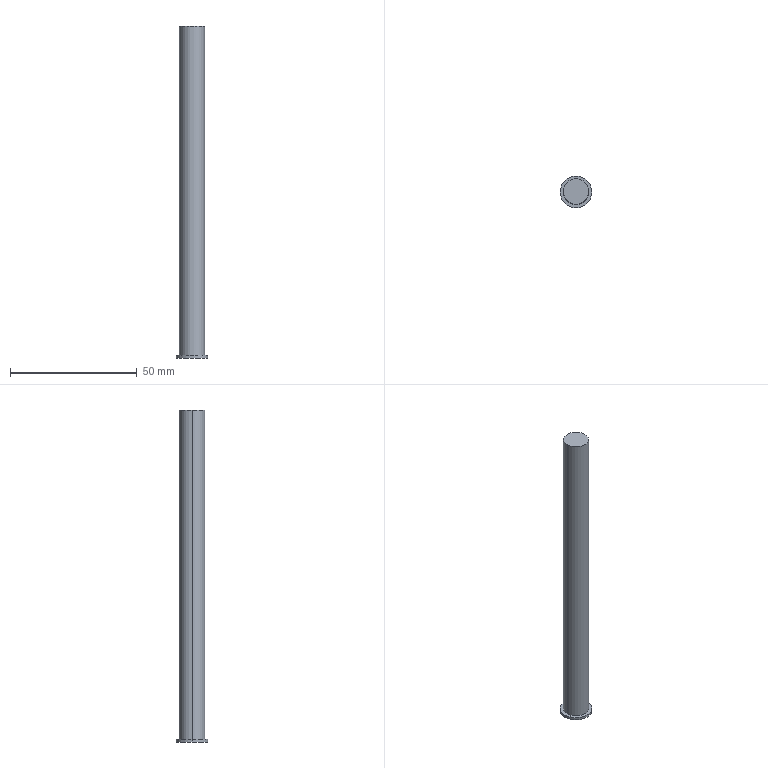Part | SolidWorks | features Extrusion 1, ICE 1 | 1 solid | 7 faces | box 12.5 x 12.5 x 131 mm | volume 10333 mm3 | cylinder 4 | plane 3 | commonest cylinder face diameters 10 x2 12.5 x2
STEP:
#1=CARTESIAN_POINT('',(-6.25,0.,-1.));
#2=VERTEX_POINT('',#1);
#3=CARTESIAN_POINT('',(6.25,0.,-1.));
#4=VERTEX_POINT('',#3);
#5=CARTESIAN_POINT('',(0.,0.,-1.));
#6=DIRECTION('',(0.,0.,-1.));
#7=DIRECTION('',(-1.,0.,0.));
#8=AXIS2_PLACEMENT_3D('',#5,#6,#7);
#9=CIRCLE('',#8,6.25);
#10=EDGE_CURVE('',#2,#4,#9,.T.);
#11=ORIENTED_EDGE('',*,*,#10,.F.);
#12=CARTESIAN_POINT('',(-6.25,0.,0.));
#13=VERTEX_POINT('',#12);
#14=CARTESIAN_POINT('',(-6.25,0.,-1.));
#15=DIRECTION('',(0.,0.,1.));
#16=VECTOR('',#15,1000.);
#17=LINE('',#14,#16);
#18=EDGE_CURVE('',#2,#13,#17,.T.);
#19=ORIENTED_EDGE('',*,*,#18,.T.);
#20=CARTESIAN_POINT('',(6.25,0.,0.));
#21=VERTEX_POINT('',#20);
#22=CARTESIAN_POINT('',(0.,0.,0.));
#23=DIRECTION('',(0.,0.,-1.));
#24=DIRECTION('',(-1.,0.,0.));
#25=AXIS2_PLACEMENT_3D('',#22,#23,#24);
#26=CIRCLE('',#25,6.25);
#27=EDGE_CURVE('',#13,#21,#26,.T.);
#28=ORIENTED_EDGE('',*,*,#27,.T.);
#29=CARTESIAN_POINT('',(6.25,0.,-1.));
#30=DIRECTION('',(0.,0.,1.));
#31=VECTOR('',#30,1000.);
#32=LINE('',#29,#31);
#33=EDGE_CURVE('',#4,#21,#32,.T.);
#34=ORIENTED_EDGE('',*,*,#33,.F.);
#35=EDGE_LOOP('',(#11,#19,#28,#34));
#36=FACE_OUTER_BOUND('',#35,.T.);
#37=CARTESIAN_POINT('',(0.,0.,-1.));
#38=DIRECTION('',(0.,0.,1.));
#39=DIRECTION('',(1.,0.,0.));
#40=AXIS2_PLACEMENT_3D('',#37,#38,#39);
#41=CYLINDRICAL_SURFACE('',#40,6.25);
#42=ADVANCED_FACE('',(#36),#41,.T.);
#43=CARTESIAN_POINT('',(5.,0.,130.));
#44=VERTEX_POINT('',#43);
#45=CARTESIAN_POINT('',(-5.,0.,130.));
#46=VERTEX_POINT('',#45);
#47=CARTESIAN_POINT('',(0.,0.,130.));
#48=DIRECTION('',(0.,0.,1.));
#49=DIRECTION('',(1.,0.,0.));
#50=AXIS2_PLACEMENT_3D('',#47,#48,#49);
#51=CIRCLE('',#50,5.);
#52=EDGE_CURVE('',#44,#46,#51,.T.);
#53=ORIENTED_EDGE('',*,*,#52,.F.);
#54=CARTESIAN_POINT('',(5.,0.,0.));
#55=VERTEX_POINT('',#54);
#56=CARTESIAN_POINT('',(5.,0.,130.));
#57=DIRECTION('',(0.,0.,-1.));
#58=VECTOR('',#57,1000.);
#59=LINE('',#56,#58);
#60=EDGE_CURVE('',#44,#55,#59,.T.);
#61=ORIENTED_EDGE('',*,*,#60,.T.);
#62=CARTESIAN_POINT('',(-5.,0.,0.));
#63=VERTEX_POINT('',#62);
#64=CARTESIAN_POINT('',(0.,0.,0.));
#65=DIRECTION('',(0.,0.,1.));
#66=DIRECTION('',(1.,0.,0.));
#67=AXIS2_PLACEMENT_3D('',#64,#65,#66);
#68=CIRCLE('',#67,5.);
#69=EDGE_CURVE('',#55,#63,#68,.T.);
#70=ORIENTED_EDGE('',*,*,#69,.T.);
#71=CARTESIAN_POINT('',(-5.,0.,130.));
#72=DIRECTION('',(0.,0.,-1.));
#73=VECTOR('',#72,1000.);
#74=LINE('',#71,#73);
#75=EDGE_CURVE('',#46,#63,#74,.T.);
#76=ORIENTED_EDGE('',*,*,#75,.F.);
#77=EDGE_LOOP('',(#53,#61,#70,#76));
#78=FACE_OUTER_BOUND('',#77,.T.);
#79=CARTESIAN_POINT('',(0.,0.,130.));
#80=DIRECTION('',(0.,0.,-1.));
#81=DIRECTION('',(-1.,0.,0.));
#82=AXIS2_PLACEMENT_3D('',#79,#80,#81);
#83=CYLINDRICAL_SURFACE('',#82,5.);
#84=ADVANCED_FACE('',(#78),#83,.T.);
#85=ORIENTED_EDGE('',*,*,#60,.F.);
#86=CARTESIAN_POINT('',(0.,0.,130.));
#87=DIRECTION('',(0.,0.,1.));
#88=DIRECTION('',(1.,0.,0.));
#89=AXIS2_PLACEMENT_3D('',#86,#87,#88);
#90=CIRCLE('',#89,5.);
#91=EDGE_CURVE('',#46,#44,#90,.T.);
#92=ORIENTED_EDGE('',*,*,#91,.F.);
#93=ORIENTED_EDGE('',*,*,#75,.T.);
#94=CARTESIAN_POINT('',(0.,0.,0.));
#95=DIRECTION('',(0.,0.,1.));
#96=DIRECTION('',(1.,0.,0.));
#97=AXIS2_PLACEMENT_3D('',#94,#95,#96);
#98=CIRCLE('',#97,5.);
#99=EDGE_CURVE('',#63,#55,#98,.T.);
#100=ORIENTED_EDGE('',*,*,#99,.T.);
#101=EDGE_LOOP('',(#85,#92,#93,#100));
#102=FACE_OUTER_BOUND('',#101,.T.);
#103=CARTESIAN_POINT('',(0.,0.,130.));
#104=DIRECTION('',(0.,0.,-1.));
#105=DIRECTION('',(-1.,0.,0.));
#106=AXIS2_PLACEMENT_3D('',#103,#104,#105);
#107=CYLINDRICAL_SURFACE('',#106,5.);
#108=ADVANCED_FACE('',(#102),#107,.T.);
#109=ORIENTED_EDGE('',*,*,#91,.T.);
#110=ORIENTED_EDGE('',*,*,#52,.T.);
#111=EDGE_LOOP('',(#109,#110));
#112=FACE_OUTER_BOUND('',#111,.T.);
#113=CARTESIAN_POINT('',(0.,0.,130.));
#114=DIRECTION('',(0.,0.,1.));
#115=DIRECTION('',(1.,0.,0.));
#116=AXIS2_PLACEMENT_3D('',#113,#114,#115);
#117=PLANE('',#116);
#118=ADVANCED_FACE('',(#112),#117,.T.);
#119=ORIENTED_EDGE('',*,*,#18,.F.);
#120=CARTESIAN_POINT('',(0.,0.,-1.));
#121=DIRECTION('',(0.,0.,-1.));
#122=DIRECTION('',(-1.,0.,0.));
#123=AXIS2_PLACEMENT_3D('',#120,#121,#122);
#124=CIRCLE('',#123,6.25);
#125=EDGE_CURVE('',#4,#2,#124,.T.);
#126=ORIENTED_EDGE('',*,*,#125,.F.);
#127=ORIENTED_EDGE('',*,*,#33,.T.);
#128=CARTESIAN_POINT('',(0.,0.,0.));
#129=DIRECTION('',(0.,0.,-1.));
#130=DIRECTION('',(-1.,0.,0.));
#131=AXIS2_PLACEMENT_3D('',#128,#129,#130);
#132=CIRCLE('',#131,6.25);
#133=EDGE_CURVE('',#21,#13,#132,.T.);
#134=ORIENTED_EDGE('',*,*,#133,.T.);
#135=EDGE_LOOP('',(#119,#126,#127,#134));
#136=FACE_OUTER_BOUND('',#135,.T.);
#137=CARTESIAN_POINT('',(0.,0.,-1.));
#138=DIRECTION('',(0.,0.,1.));
#139=DIRECTION('',(1.,0.,0.));
#140=AXIS2_PLACEMENT_3D('',#137,#138,#139);
#141=CYLINDRICAL_SURFACE('',#140,6.25);
#142=ADVANCED_FACE('',(#136),#141,.T.);
#143=ORIENTED_EDGE('',*,*,#125,.T.);
#144=ORIENTED_EDGE('',*,*,#10,.T.);
#145=EDGE_LOOP('',(#143,#144));
#146=FACE_OUTER_BOUND('',#145,.T.);
#147=CARTESIAN_POINT('',(0.,0.,-1.));
#148=DIRECTION('',(0.,0.,-1.));
#149=DIRECTION('',(-1.,0.,0.));
#150=AXIS2_PLACEMENT_3D('',#147,#148,#149);
#151=PLANE('',#150);
#152=ADVANCED_FACE('',(#146),#151,.T.);
#153=ORIENTED_EDGE('',*,*,#99,.F.);
#154=ORIENTED_EDGE('',*,*,#69,.F.);
#155=EDGE_LOOP('',(#153,#154));
#156=FACE_BOUND('',#155,.T.);
#157=ORIENTED_EDGE('',*,*,#133,.F.);
#158=ORIENTED_EDGE('',*,*,#27,.F.);
#159=EDGE_LOOP('',(#157,#158));
#160=FACE_OUTER_BOUND('',#159,.T.);
#161=CARTESIAN_POINT('',(0.,0.,0.));
#162=DIRECTION('',(0.,0.,-1.));
#163=DIRECTION('',(-1.,0.,0.));
#164=AXIS2_PLACEMENT_3D('',#161,#162,#163);
#165=PLANE('',#164);
#166=ADVANCED_FACE('',(#156,#160),#165,.F.);
#167=CLOSED_SHELL('',(#42,#84,#108,#118,#142,#152,#166));
#168=MANIFOLD_SOLID_BREP('',#167);
#169=CARTESIAN_POINT('',(0.,0.,0.));
#170=DIRECTION('',(0.,0.,1.));
#171=DIRECTION('',(1.,0.,0.));
#172=AXIS2_PLACEMENT_3D('',#169,#170,#171);
#173=(LENGTH_UNIT()NAMED_UNIT(*)SI_UNIT(.MILLI.,.METRE.));
#174=UNCERTAINTY_MEASURE_WITH_UNIT(LENGTH_MEASURE(0.00001),#173,'','');
#175=(NAMED_UNIT(*)PLANE_ANGLE_UNIT()SI_UNIT($,.RADIAN.));
#176=(NAMED_UNIT(*)SI_UNIT($,.STERADIAN.)SOLID_ANGLE_UNIT());
#177=(GEOMETRIC_REPRESENTATION_CONTEXT(3)GLOBAL_UNCERTAINTY_ASSIGNED_CONTEXT((#174))GLOBAL_UNIT_ASSIGNED_CONTEXT((#173,#175,#176))REPRESENTATION_CONTEXT('',''));
#178=ADVANCED_BREP_SHAPE_REPRESENTATION('',(#168,#172),#177);